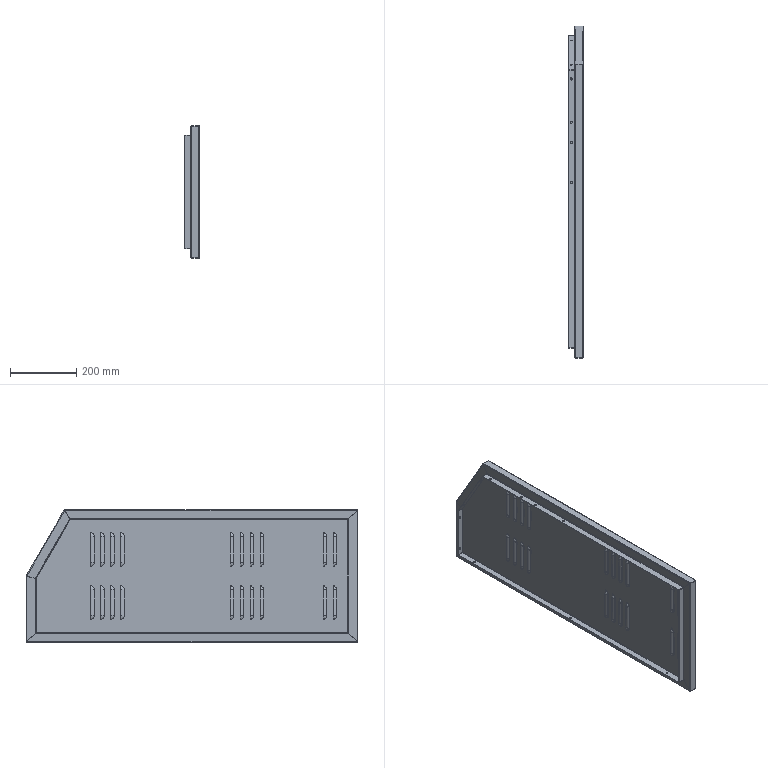Part | SolidWorks | features Cut 3, EdgeFlange 3, FormToolInstance 3, ICE 2, FlatPattern 1, Fold 1, SMBaseFlange 1, SheetMetal 1, UnFold 1 | 1 solid | 529 faces | box 43.8 x 1000 x 400 mm | volume 684379 mm3 | torus 160 | plane 137 | cylinder 132 | spline 100 | commonest cylinder face diameters 3.6 x20 6 x20 29 x20 31.4 x20 6.5 x16 2 x15